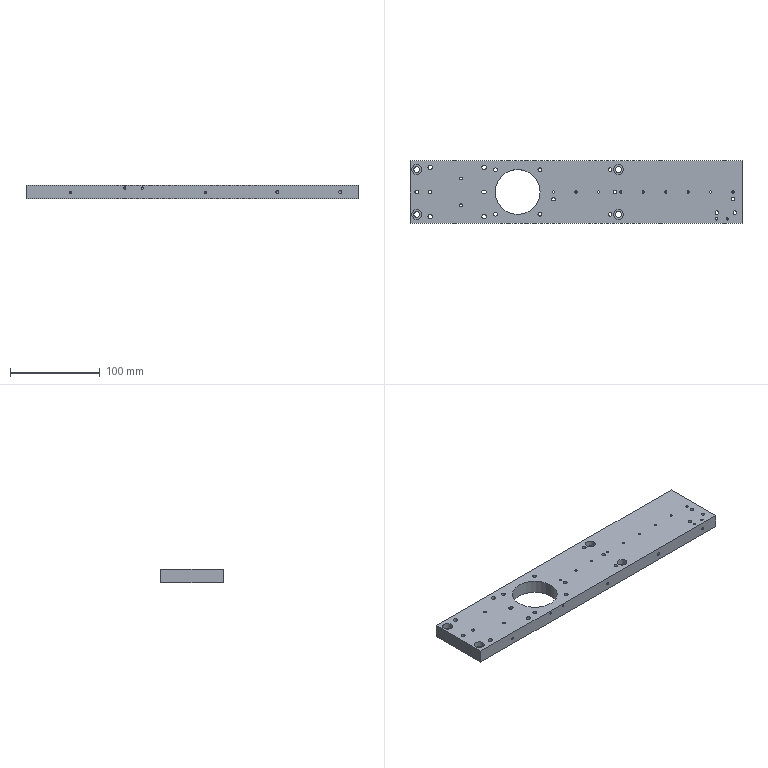CAM job | NX | 3-axis milling, drilling | part box 370 x 70 x 15 mm | stock box 370 x 70 x 15 mm
Tools:
number,name,description,diameter,corner_radius,flute_length,length,flutes
3,D3,平底铣刀-粗,3.0,0.0,20.0,75.0,2
6,D6,平底铣刀-粗,6.0,0.0,25.0,75.0,2
9,D10,平底铣刀-粗,10.0,0.0,35.0,75.0,2
11,D3-J,平底铣刀-精,3.0,0.0,50.0,75.0,2
7,D6-J,平底铣刀-精,6.0,0.0,25.0,75.0,2
10,D10-J,平底铣刀-精,10.0,0.0,35.0,75.0,2
2,D6倒角刀,倒角刀,6.0,0.0,3.0,25.0,2
20,M3X0.5,丝锥,2.5,0.0,35.0,50.0,2
21,M4X0.7,丝锥,3.3,0.0,35.0,50.0,2
22,M5X0.8,丝锥,4.2,0.0,35.0,50.0,2
23,M6X1.0,丝锥,5.0,0.0,35.0,50.0,2
19,D4铰刀,Drilling Tool,4.0,0.0,75.0,100.0,6
1,C6定点钻,倒角刀,6.0,0.0,3.0,3.0,2
12,ZT2.6,钻头,2.6,0.0,35.0,50.0,2
13,ZT3.4,钻头,3.4,0.0,35.0,50.0,2
15,ZT5.1,钻头,5.1,0.0,35.0,50.0,2
18,ZT6.6,钻头,6.6,0.0,35.0,50.0,2
18,钻头6.6,Drilling Tool,6.6,0.0,35.0,50.0,2
17,ZT3.9,Drilling Tool,3.9,0.0,35.0,50.0,2
14,ZT4.3,Drilling Tool,4.3,0.0,50.0,75.0,4
Operations:
program,operation,operation_type,tool,method,geometry_group,spindle_rpm,surface_speed,feed_per_tooth,feed_cut,feed_plunge,cut_length_mm,path_length_mm,cut_time_min,machine_time_min
B,DRILL-CHAMFER_4,Operation,D6倒角刀,METHOD,W-B,2000.0,0.0,0.025,100.0,0.0,52.25,419.147,0.5225,0.5592
B,DRILL-CHAMFER_5,Operation,D6倒角刀,METHOD,W-B,2000.0,0.0,0.025,100.0,0.0,10.4,93.95,0.104,0.1124
B,DRILL-CHAMFER_6,Operation,D6倒角刀,METHOD,W-B,2000.0,0.0,0.025,100.0,0.0,47.7,589.897,0.477,0.5312
B,DRILL-CHAMFER_7,Operation,D6倒角刀,METHOD,W-B,2000.0,0.0,0.025,100.0,0.0,22.8,243.365,0.228,0.2501
B,MILL-CHAMFER_5,PlanarMilling,D6倒角刀,METHOD,W-B,4000.0,75.398,0.0375,300.0,100.0,72.081,410.897,0.2403,0.2742
B,MILL-CHAMFER_6,PlanarMilling,D6倒角刀,METHOD,W-B,4000.0,75.398,0.075,600.0,100.0,77.764,571.572,0.1296,0.179
B,C0.3封闭铣廓倒角6X45L_COPY_1,PlanarMilling,D6倒角刀,爬面_倒角-切深0-步距G,W-B,4000.0,75.398,0.125,1000.0,100.0,1086.433,1403.586,1.086,1.118
A,型腔铣开粗-中_COPY,CavityMilling,D10,分层开粗-切深K-步距G,W-A,3000.0,94.248,0.4167,2500.0,100.0,21818.948,23385.714,8.728,8.97
A,打点0.8,Operation,C6定点钻,METHOD,W-A,3000.0,56.549,0.01,60.0,0.0,3.6,86.213,0.06,0.0683
A,打点-深0.8,Operation,C6定点钻,NONE,W-A,3000.0,56.0,0.01,60.0,90.0,61.2,925.667,1.02,1.106
A,通孔-M3螺纹底孔,Operation,ZT2.6,NONE,W-A,1500.0,11.781,0.02,60.0,90.0,220.0,732.914,3.667,3.718
A,通孔-M4螺纹底孔,Operation,ZT3.4,NONE,W-A,1500.0,15.551,0.02,60.0,90.0,42.0,155.017,0.7,0.7113
A,通孔-精孔4.0预钻,Operation,ZT3.9,NONE,W-A,1500.0,18.378,0.0167,50.0,90.0,201.258,955.366,4.025,4.101
A,通孔-M5螺纹底孔,Operation,ZT4.3,NONE,W-A,1200.0,15.834,0.0333,80.0,90.0,84.0,359.523,1.05,1.078
A,通孔-M6螺纹底孔,Operation,ZT5.1,NONE,W-A,800.0,12.566,0.0625,100.0,90.0,88.0,389.026,0.88,0.9101
A,沉头孔-钻孔0段,Operation,钻头6.6,NONE,W-A,600.0,12.441,0.1,120.0,90.0,79.621,527.264,0.6635,0.7083
A,通孔-10-12.5,Operation,ZT6.6,NONE,W-A,500.0,78.54,0.12,120.0,90.0,19.983,79.966,0.1665,0.1725
A,通腰槽粗_1,VolumeBased25DMillingOperation,D3,METHOD,W-A,3500.0,32.987,0.0714,500.0,100.0,523.111,577.111,1.046,1.052
A,铣孔开粗D6_1,CylinderMilling,D6,NONE,W-A,4000.0,75.398,0.25,2000.0,100.0,2171.652,2680.252,1.086,1.137
A,铣孔精光D6_1,CylinderMilling,D6-J,精光步距切深关,W-A,4000.0,75.398,0.1,800.0,100.0,178.461,689.061,0.2231,0.2741
A,DRILL-CHAMFER_1,Operation,D6倒角刀,METHOD,W-A,4000.0,75.398,0.01,80.0,0.0,52.25,419.147,0.6531,0.6898
A,DRILL-CHAMFER_2,Operation,D6倒角刀,METHOD,W-A,4000.0,75.398,0.01,80.0,0.0,10.4,93.95,0.13,0.1384
A,DRILL-CHAMFER_3,Operation,D6倒角刀,METHOD,W-A,4000.0,75.398,0.01,80.0,0.0,47.7,589.897,0.5962,0.6505
A,MILL-CHAMFER_1,PlanarMilling,D6倒角刀,METHOD,W-A,4000.0,75.398,0.025,200.0,100.0,72.081,384.593,0.3604,0.3917
A,MILL-CHAMFER_2,PlanarMilling,D6倒角刀,METHOD,W-A,4000.0,75.398,0.0375,300.0,100.0,79.753,414.587,0.2658,0.2993
A,MILL-CHAMFER_3,PlanarMilling,D6倒角刀,NONE,W-A,4000.0,75.398,0.1,800.0,100.0,173.57,650.329,0.217,0.2646
A,MILL-CHAMFER_4,PlanarMilling,D6倒角刀,METHOD,W-A,4000.0,75.398,0.1,800.0,100.0,163.106,204.106,0.2039,0.208
A,C0.3封闭铣廓倒角6X45L_COPY,PlanarMilling,D6倒角刀,爬面_倒角-切深0-步距G,W-A,4000.0,75.398,0.125,1000.0,100.0,898.958,935.158,0.899,0.9026
A,C0.3封闭铣廓倒角6X45L_COPY_COPY,PlanarMilling,D6倒角刀,爬面_倒角-切深0-步距G,W-A,4000.0,75.398,0.075,600.0,100.0,23.401,59.401,0.039,0.0426
A,REAMING,Operation,D4铰刀,METHOD,W-A,500.0,6.283,0.0167,50.0,0.0,153.0,783.343,3.06,3.123
A,通孔-攻牙M3.,Operation,M3X0.5,METHOD,W-A,600.0,4.712,0.0004,0.5,90.0,203.5,699.914,407.0,407.05
A,通孔-攻牙M4,Operation,M4X0.7,METHOD,W-A,500.0,5.184,0.0007,0.7,90.0,39.0,149.017,55.714,55.725
A,通孔-攻牙M5,Operation,M5X0.8,METHOD,W-A,500.0,6.597,0.0008,0.8,90.0,78.0,347.523,97.5,97.527
A,通孔-攻牙M6,Operation,M6X1.0,METHOD,W-A,400.0,6.283,0.0013,1.0,90.0,78.0,369.026,78.0,78.029
A,底壁铣精光侧面-中_COPY,VolumeBased25DMillingOperation,D10-J,侧刃精光-切深K-步距G,W-A,3000.0,94.245,0.1333,800.0,100.0,268.784,317.483,0.336,0.3409
A,腰槽精_1,VolumeBased25DMillingOperation,D3-J,METHOD,W-A,3700.0,32.0,0.027,200.0,100.0,30.424,126.382,0.1521,0.1617